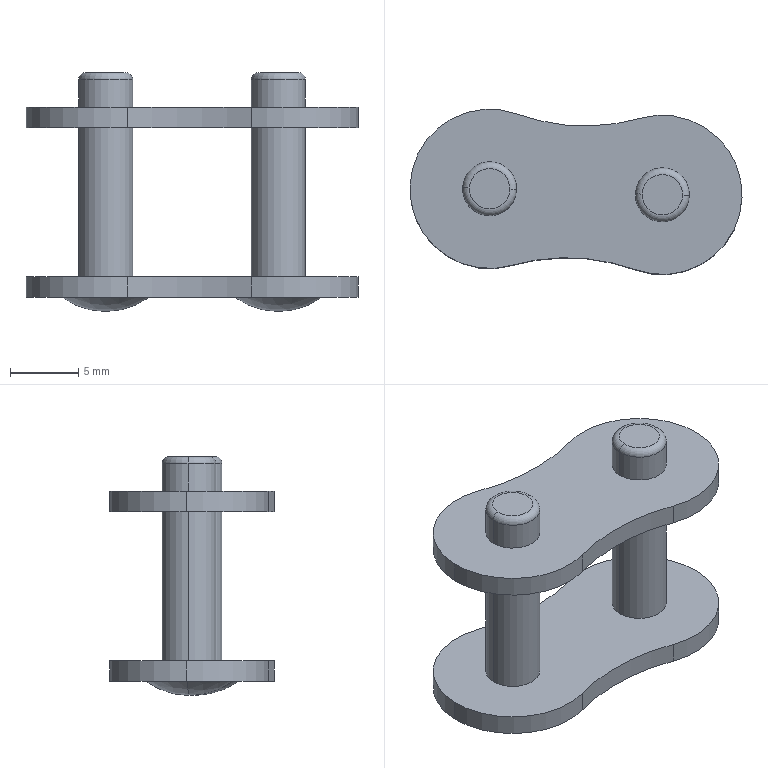Part | STEP file | CHES40-46-Part-10 | 1 solid | 32 faces | box 24.392 x 12.143 x 17.55 mm | volume 1093 mm3 | cylinder 18 | plane 6 | torus 4 | sphere 4 | commonest cylinder face diameters 3.97 x8 11.7 x6 29.64 x4
STEP:
#1=CARTESIAN_POINT('',(-138.255,-2.268,9.53));
#2=VERTEX_POINT('',#1);
#3=CARTESIAN_POINT('',(-141.223,-2.164,9.53));
#4=VERTEX_POINT('',#3);
#5=CARTESIAN_POINT('',(-139.739,-2.216,9.53));
#6=DIRECTION('',(0.,0.,1.));
#7=DIRECTION('',(-0.9994,0.0349,0.));
#8=AXIS2_PLACEMENT_3D('',#5,#6,#7);
#9=CIRCLE('',#8,1.485);
#10=EDGE_CURVE('',#2,#4,#9,.T.);
#11=ORIENTED_EDGE('',*,*,#10,.F.);
#12=CARTESIAN_POINT('',(-137.755,-2.285,9.03));
#13=VERTEX_POINT('',#12);
#14=CARTESIAN_POINT('',(-138.255,-2.268,9.03));
#15=DIRECTION('',(0.0349,0.9994,0.));
#16=DIRECTION('',(-0.9994,0.0349,0.));
#17=AXIS2_PLACEMENT_3D('',#14,#15,#16);
#18=CIRCLE('',#17,0.5);
#19=EDGE_CURVE('',#2,#13,#18,.T.);
#20=ORIENTED_EDGE('',*,*,#19,.T.);
#21=CARTESIAN_POINT('',(-141.722,-2.147,9.03));
#22=VERTEX_POINT('',#21);
#23=CARTESIAN_POINT('',(-139.739,-2.216,9.03));
#24=DIRECTION('',(0.,0.,-1.));
#25=DIRECTION('',(-0.9994,0.0349,0.));
#26=AXIS2_PLACEMENT_3D('',#23,#24,#25);
#27=CIRCLE('',#26,1.985);
#28=EDGE_CURVE('',#22,#13,#27,.T.);
#29=ORIENTED_EDGE('',*,*,#28,.F.);
#30=CARTESIAN_POINT('',(-141.223,-2.164,9.03));
#31=DIRECTION('',(-0.0349,-0.9994,0.));
#32=DIRECTION('',(0.9994,-0.0349,0.));
#33=AXIS2_PLACEMENT_3D('',#30,#31,#32);
#34=CIRCLE('',#33,0.5);
#35=EDGE_CURVE('',#4,#22,#34,.T.);
#36=ORIENTED_EDGE('',*,*,#35,.F.);
#37=EDGE_LOOP('',(#11,#20,#29,#36));
#38=FACE_OUTER_BOUND('',#37,.T.);
#39=CARTESIAN_POINT('',(-139.739,-2.216,9.03));
#40=DIRECTION('',(0.,0.,-1.));
#41=DIRECTION('',(-0.9994,0.0349,0.));
#42=AXIS2_PLACEMENT_3D('',#39,#40,#41);
#43=TOROIDAL_SURFACE('',#42,1.485,0.5);
#44=ADVANCED_FACE('',(#38),#43,.T.);
#45=CARTESIAN_POINT('',(-125.562,-2.711,9.53));
#46=VERTEX_POINT('',#45);
#47=CARTESIAN_POINT('',(-128.531,-2.608,9.53));
#48=VERTEX_POINT('',#47);
#49=CARTESIAN_POINT('',(-127.046,-2.659,9.53));
#50=DIRECTION('',(0.,0.,1.));
#51=DIRECTION('',(-0.9994,0.0349,0.));
#52=AXIS2_PLACEMENT_3D('',#49,#50,#51);
#53=CIRCLE('',#52,1.485);
#54=EDGE_CURVE('',#46,#48,#53,.T.);
#55=ORIENTED_EDGE('',*,*,#54,.F.);
#56=CARTESIAN_POINT('',(-125.063,-2.729,9.03));
#57=VERTEX_POINT('',#56);
#58=CARTESIAN_POINT('',(-125.562,-2.711,9.03));
#59=DIRECTION('',(0.0349,0.9994,0.));
#60=DIRECTION('',(-0.9994,0.0349,0.));
#61=AXIS2_PLACEMENT_3D('',#58,#59,#60);
#62=CIRCLE('',#61,0.5);
#63=EDGE_CURVE('',#46,#57,#62,.T.);
#64=ORIENTED_EDGE('',*,*,#63,.T.);
#65=CARTESIAN_POINT('',(-129.03,-2.59,9.03));
#66=VERTEX_POINT('',#65);
#67=CARTESIAN_POINT('',(-127.046,-2.659,9.03));
#68=DIRECTION('',(0.,0.,-1.));
#69=DIRECTION('',(-0.9994,0.0349,0.));
#70=AXIS2_PLACEMENT_3D('',#67,#68,#69);
#71=CIRCLE('',#70,1.985);
#72=EDGE_CURVE('',#66,#57,#71,.T.);
#73=ORIENTED_EDGE('',*,*,#72,.F.);
#74=CARTESIAN_POINT('',(-128.531,-2.608,9.03));
#75=DIRECTION('',(-0.0349,-0.9994,0.));
#76=DIRECTION('',(0.9994,-0.0349,0.));
#77=AXIS2_PLACEMENT_3D('',#74,#75,#76);
#78=CIRCLE('',#77,0.5);
#79=EDGE_CURVE('',#48,#66,#78,.T.);
#80=ORIENTED_EDGE('',*,*,#79,.F.);
#81=EDGE_LOOP('',(#55,#64,#73,#80));
#82=FACE_OUTER_BOUND('',#81,.T.);
#83=CARTESIAN_POINT('',(-127.046,-2.659,9.03));
#84=DIRECTION('',(0.,0.,-1.));
#85=DIRECTION('',(-0.9994,0.0349,0.));
#86=AXIS2_PLACEMENT_3D('',#83,#84,#85);
#87=TOROIDAL_SURFACE('',#86,1.485,0.5);
#88=ADVANCED_FACE('',(#82),#87,.T.);
#89=CARTESIAN_POINT('',(-142.937,-2.104,-6.975));
#90=VERTEX_POINT('',#89);
#91=CARTESIAN_POINT('',(-136.541,-2.328,-6.975));
#92=VERTEX_POINT('',#91);
#93=CARTESIAN_POINT('',(-139.739,-2.216,-6.975));
#94=DIRECTION('',(0.,0.,1.));
#95=DIRECTION('',(0.9994,-0.0349,0.));
#96=AXIS2_PLACEMENT_3D('',#93,#94,#95);
#97=CIRCLE('',#96,3.2);
#98=EDGE_CURVE('',#90,#92,#97,.T.);
#99=ORIENTED_EDGE('',*,*,#98,.F.);
#100=CARTESIAN_POINT('',(-139.739,-2.216,-8.02));
#101=VERTEX_POINT('',#100);
#102=CARTESIAN_POINT('',(-139.739,-2.216,-2.598));
#103=DIRECTION('',(-0.0349,-0.9994,0.));
#104=DIRECTION('',(0.9994,-0.0349,0.));
#105=AXIS2_PLACEMENT_3D('',#102,#103,#104);
#106=CIRCLE('',#105,5.422);
#107=EDGE_CURVE('',#90,#101,#106,.T.);
#108=ORIENTED_EDGE('',*,*,#107,.T.);
#109=CARTESIAN_POINT('',(-139.739,-2.216,-2.598));
#110=DIRECTION('',(0.0349,0.9994,0.));
#111=DIRECTION('',(-0.9994,0.0349,0.));
#112=AXIS2_PLACEMENT_3D('',#109,#110,#111);
#113=CIRCLE('',#112,5.422);
#114=EDGE_CURVE('',#92,#101,#113,.T.);
#115=ORIENTED_EDGE('',*,*,#114,.F.);
#116=EDGE_LOOP('',(#99,#108,#115));
#117=FACE_OUTER_BOUND('',#116,.T.);
#118=CARTESIAN_POINT('',(-139.739,-2.216,-2.598));
#119=DIRECTION('',(-0.0349,-0.9994,0.));
#120=DIRECTION('',(0.9994,-0.0349,0.));
#121=AXIS2_PLACEMENT_3D('',#118,#119,#120);
#122=SPHERICAL_SURFACE('',#121,5.422);
#123=ADVANCED_FACE('',(#117),#122,.T.);
#124=CARTESIAN_POINT('',(-130.244,-2.548,-6.975));
#125=VERTEX_POINT('',#124);
#126=CARTESIAN_POINT('',(-123.848,-2.771,-6.975));
#127=VERTEX_POINT('',#126);
#128=CARTESIAN_POINT('',(-127.046,-2.659,-6.975));
#129=DIRECTION('',(0.,0.,1.));
#130=DIRECTION('',(0.9994,-0.0349,0.));
#131=AXIS2_PLACEMENT_3D('',#128,#129,#130);
#132=CIRCLE('',#131,3.2);
#133=EDGE_CURVE('',#125,#127,#132,.T.);
#134=ORIENTED_EDGE('',*,*,#133,.F.);
#135=CARTESIAN_POINT('',(-127.046,-2.659,-8.02));
#136=VERTEX_POINT('',#135);
#137=CARTESIAN_POINT('',(-127.046,-2.659,-2.598));
#138=DIRECTION('',(-0.0349,-0.9994,0.));
#139=DIRECTION('',(0.9994,-0.0349,0.));
#140=AXIS2_PLACEMENT_3D('',#137,#138,#139);
#141=CIRCLE('',#140,5.422);
#142=EDGE_CURVE('',#125,#136,#141,.T.);
#143=ORIENTED_EDGE('',*,*,#142,.T.);
#144=CARTESIAN_POINT('',(-127.046,-2.659,-2.598));
#145=DIRECTION('',(0.0349,0.9994,0.));
#146=DIRECTION('',(-0.9994,0.0349,0.));
#147=AXIS2_PLACEMENT_3D('',#144,#145,#146);
#148=CIRCLE('',#147,5.422);
#149=EDGE_CURVE('',#127,#136,#148,.T.);
#150=ORIENTED_EDGE('',*,*,#149,.F.);
#151=EDGE_LOOP('',(#134,#143,#150));
#152=FACE_OUTER_BOUND('',#151,.T.);
#153=CARTESIAN_POINT('',(-127.046,-2.659,-2.598));
#154=DIRECTION('',(-0.0349,-0.9994,0.));
#155=DIRECTION('',(0.9994,-0.0349,0.));
#156=AXIS2_PLACEMENT_3D('',#153,#154,#155);
#157=SPHERICAL_SURFACE('',#156,5.422);
#158=ADVANCED_FACE('',(#152),#157,.T.);
#159=CARTESIAN_POINT('',(-145.585,-2.012,-5.475));
#160=VERTEX_POINT('',#159);
#161=CARTESIAN_POINT('',(-138.137,-7.843,-5.475));
#162=VERTEX_POINT('',#161);
#163=CARTESIAN_POINT('',(-139.739,-2.216,-5.475));
#164=DIRECTION('',(0.,0.,1.));
#165=DIRECTION('',(0.9994,-0.0349,0.));
#166=AXIS2_PLACEMENT_3D('',#163,#164,#165);
#167=CIRCLE('',#166,5.85);
#168=EDGE_CURVE('',#160,#162,#167,.T.);
#169=ORIENTED_EDGE('',*,*,#168,.F.);
#170=CARTESIAN_POINT('',(-145.585,-2.012,-6.975));
#171=VERTEX_POINT('',#170);
#172=CARTESIAN_POINT('',(-145.585,-2.012,-5.475));
#173=DIRECTION('',(0.,0.,-1.));
#174=VECTOR('',#173,1000.);
#175=LINE('',#172,#174);
#176=EDGE_CURVE('',#160,#171,#175,.T.);
#177=ORIENTED_EDGE('',*,*,#176,.T.);
#178=CARTESIAN_POINT('',(-138.137,-7.843,-6.975));
#179=VERTEX_POINT('',#178);
#180=CARTESIAN_POINT('',(-139.739,-2.216,-6.975));
#181=DIRECTION('',(0.,0.,1.));
#182=DIRECTION('',(0.9994,-0.0349,0.));
#183=AXIS2_PLACEMENT_3D('',#180,#181,#182);
#184=CIRCLE('',#183,5.85);
#185=EDGE_CURVE('',#171,#179,#184,.T.);
#186=ORIENTED_EDGE('',*,*,#185,.T.);
#187=CARTESIAN_POINT('',(-138.137,-7.843,-5.475));
#188=DIRECTION('',(0.,0.,-1.));
#189=VECTOR('',#188,1000.);
#190=LINE('',#187,#189);
#191=EDGE_CURVE('',#162,#179,#190,.T.);
#192=ORIENTED_EDGE('',*,*,#191,.F.);
#193=EDGE_LOOP('',(#169,#177,#186,#192));
#194=FACE_OUTER_BOUND('',#193,.T.);
#195=CARTESIAN_POINT('',(-139.739,-2.216,-5.475));
#196=DIRECTION('',(0.,0.,-1.));
#197=DIRECTION('',(-0.9994,0.0349,0.));
#198=AXIS2_PLACEMENT_3D('',#195,#196,#197);
#199=CYLINDRICAL_SURFACE('',#198,5.85);
#200=ADVANCED_FACE('',(#194),#199,.T.);
#201=CARTESIAN_POINT('',(-129.03,-2.59,5.475));
#202=VERTEX_POINT('',#201);
#203=CARTESIAN_POINT('',(-125.063,-2.729,5.475));
#204=VERTEX_POINT('',#203);
#205=CARTESIAN_POINT('',(-127.046,-2.659,5.475));
#206=DIRECTION('',(0.,0.,-1.));
#207=DIRECTION('',(-0.9994,0.0349,0.));
#208=AXIS2_PLACEMENT_3D('',#205,#206,#207);
#209=CIRCLE('',#208,1.985);
#210=EDGE_CURVE('',#202,#204,#209,.T.);
#211=ORIENTED_EDGE('',*,*,#210,.T.);
#212=CARTESIAN_POINT('',(-125.063,-2.729,-5.475));
#213=VERTEX_POINT('',#212);
#214=CARTESIAN_POINT('',(-125.063,-2.729,-8.02));
#215=DIRECTION('',(0.,0.,-1.));
#216=VECTOR('',#215,1000.);
#217=LINE('',#214,#216);
#218=EDGE_CURVE('',#204,#213,#217,.T.);
#219=ORIENTED_EDGE('',*,*,#218,.T.);
#220=CARTESIAN_POINT('',(-129.03,-2.59,-5.475));
#221=VERTEX_POINT('',#220);
#222=CARTESIAN_POINT('',(-127.046,-2.659,-5.475));
#223=DIRECTION('',(0.,0.,1.));
#224=DIRECTION('',(0.9994,-0.0349,0.));
#225=AXIS2_PLACEMENT_3D('',#222,#223,#224);
#226=CIRCLE('',#225,1.985);
#227=EDGE_CURVE('',#213,#221,#226,.T.);
#228=ORIENTED_EDGE('',*,*,#227,.T.);
#229=CARTESIAN_POINT('',(-129.03,-2.59,-8.02));
#230=DIRECTION('',(0.,0.,-1.));
#231=VECTOR('',#230,1000.);
#232=LINE('',#229,#231);
#233=EDGE_CURVE('',#202,#221,#232,.T.);
#234=ORIENTED_EDGE('',*,*,#233,.F.);
#235=EDGE_LOOP('',(#211,#219,#228,#234));
#236=FACE_OUTER_BOUND('',#235,.T.);
#237=CARTESIAN_POINT('',(-127.046,-2.659,-8.02));
#238=DIRECTION('',(0.,0.,-1.));
#239=DIRECTION('',(-0.9994,0.0349,0.));
#240=AXIS2_PLACEMENT_3D('',#237,#238,#239);
#241=CYLINDRICAL_SURFACE('',#240,1.985);
#242=ADVANCED_FACE('',(#236),#241,.T.);
#243=ORIENTED_EDGE('',*,*,#72,.T.);
#244=CARTESIAN_POINT('',(-125.063,-2.729,6.975));
#245=VERTEX_POINT('',#244);
#246=CARTESIAN_POINT('',(-125.063,-2.729,-8.02));
#247=DIRECTION('',(0.,0.,-1.));
#248=VECTOR('',#247,1000.);
#249=LINE('',#246,#248);
#250=EDGE_CURVE('',#57,#245,#249,.T.);
#251=ORIENTED_EDGE('',*,*,#250,.T.);
#252=CARTESIAN_POINT('',(-129.03,-2.59,6.975));
#253=VERTEX_POINT('',#252);
#254=CARTESIAN_POINT('',(-127.046,-2.659,6.975));
#255=DIRECTION('',(0.,0.,1.));
#256=DIRECTION('',(-0.9994,0.0349,0.));
#257=AXIS2_PLACEMENT_3D('',#254,#255,#256);
#258=CIRCLE('',#257,1.985);
#259=EDGE_CURVE('',#245,#253,#258,.T.);
#260=ORIENTED_EDGE('',*,*,#259,.T.);
#261=CARTESIAN_POINT('',(-129.03,-2.59,-8.02));
#262=DIRECTION('',(0.,0.,-1.));
#263=VECTOR('',#262,1000.);
#264=LINE('',#261,#263);
#265=EDGE_CURVE('',#66,#253,#264,.T.);
#266=ORIENTED_EDGE('',*,*,#265,.F.);
#267=EDGE_LOOP('',(#243,#251,#260,#266));
#268=FACE_OUTER_BOUND('',#267,.T.);
#269=CARTESIAN_POINT('',(-127.046,-2.659,-8.02));
#270=DIRECTION('',(0.,0.,-1.));
#271=DIRECTION('',(-0.9994,0.0349,0.));
#272=AXIS2_PLACEMENT_3D('',#269,#270,#271);
#273=CYLINDRICAL_SURFACE('',#272,1.985);
#274=ADVANCED_FACE('',(#268),#273,.T.);
#275=ORIENTED_EDGE('',*,*,#28,.T.);
#276=CARTESIAN_POINT('',(-137.755,-2.285,6.975));
#277=VERTEX_POINT('',#276);
#278=CARTESIAN_POINT('',(-137.755,-2.285,-8.02));
#279=DIRECTION('',(0.,0.,-1.));
#280=VECTOR('',#279,1000.);
#281=LINE('',#278,#280);
#282=EDGE_CURVE('',#13,#277,#281,.T.);
#283=ORIENTED_EDGE('',*,*,#282,.T.);
#284=CARTESIAN_POINT('',(-141.722,-2.147,6.975));
#285=VERTEX_POINT('',#284);
#286=CARTESIAN_POINT('',(-139.739,-2.216,6.975));
#287=DIRECTION('',(0.,0.,-1.));
#288=DIRECTION('',(-0.9994,0.0349,0.));
#289=AXIS2_PLACEMENT_3D('',#286,#287,#288);
#290=CIRCLE('',#289,1.985);
#291=EDGE_CURVE('',#285,#277,#290,.T.);
#292=ORIENTED_EDGE('',*,*,#291,.F.);
#293=CARTESIAN_POINT('',(-141.722,-2.147,-8.02));
#294=DIRECTION('',(0.,0.,-1.));
#295=VECTOR('',#294,1000.);
#296=LINE('',#293,#295);
#297=EDGE_CURVE('',#22,#285,#296,.T.);
#298=ORIENTED_EDGE('',*,*,#297,.F.);
#299=EDGE_LOOP('',(#275,#283,#292,#298));
#300=FACE_OUTER_BOUND('',#299,.T.);
#301=CARTESIAN_POINT('',(-139.739,-2.216,-8.02));
#302=DIRECTION('',(0.,0.,-1.));
#303=DIRECTION('',(-0.9994,0.0349,0.));
#304=AXIS2_PLACEMENT_3D('',#301,#302,#303);
#305=CYLINDRICAL_SURFACE('',#304,1.985);
#306=ADVANCED_FACE('',(#300),#305,.T.);
#307=CARTESIAN_POINT('',(-137.748,3.285,5.475));
#308=VERTEX_POINT('',#307);
#309=CARTESIAN_POINT('',(-145.585,-2.012,5.475));
#310=VERTEX_POINT('',#309);
#311=CARTESIAN_POINT('',(-139.739,-2.216,5.475));
#312=DIRECTION('',(0.,0.,1.));
#313=DIRECTION('',(0.9994,-0.0349,0.));
#314=AXIS2_PLACEMENT_3D('',#311,#312,#313);
#315=CIRCLE('',#314,5.85);
#316=EDGE_CURVE('',#308,#310,#315,.T.);
#317=ORIENTED_EDGE('',*,*,#316,.T.);
#318=CARTESIAN_POINT('',(-145.585,-2.012,6.975));
#319=VERTEX_POINT('',#318);
#320=CARTESIAN_POINT('',(-145.585,-2.012,5.475));
#321=DIRECTION('',(0.,0.,1.));
#322=VECTOR('',#321,1000.);
#323=LINE('',#320,#322);
#324=EDGE_CURVE('',#310,#319,#323,.T.);
#325=ORIENTED_EDGE('',*,*,#324,.T.);
#326=CARTESIAN_POINT('',(-137.748,3.285,6.975));
#327=VERTEX_POINT('',#326);
#328=CARTESIAN_POINT('',(-139.739,-2.216,6.975));
#329=DIRECTION('',(0.,0.,1.));
#330=DIRECTION('',(0.9994,-0.0349,0.));
#331=AXIS2_PLACEMENT_3D('',#328,#329,#330);
#332=CIRCLE('',#331,5.85);
#333=EDGE_CURVE('',#327,#319,#332,.T.);
#334=ORIENTED_EDGE('',*,*,#333,.F.);
#335=CARTESIAN_POINT('',(-137.748,3.285,5.475));
#336=DIRECTION('',(0.,0.,1.));
#337=VECTOR('',#336,1000.);
#338=LINE('',#335,#337);
#339=EDGE_CURVE('',#308,#327,#338,.T.);
#340=ORIENTED_EDGE('',*,*,#339,.F.);
#341=EDGE_LOOP('',(#317,#325,#334,#340));
#342=FACE_OUTER_BOUND('',#341,.T.);
#343=CARTESIAN_POINT('',(-139.739,-2.216,5.475));
#344=DIRECTION('',(0.,0.,1.));
#345=DIRECTION('',(-0.9994,0.0349,0.));
#346=AXIS2_PLACEMENT_3D('',#343,#344,#345);
#347=CYLINDRICAL_SURFACE('',#346,5.85);
#348=ADVANCED_FACE('',(#342),#347,.T.);
#349=CARTESIAN_POINT('',(-141.722,-2.147,5.475));
#350=VERTEX_POINT('',#349);
#351=CARTESIAN_POINT('',(-137.755,-2.285,5.475));
#352=VERTEX_POINT('',#351);
#353=CARTESIAN_POINT('',(-139.739,-2.216,5.475));
#354=DIRECTION('',(0.,0.,-1.));
#355=DIRECTION('',(-0.9994,0.0349,0.));
#356=AXIS2_PLACEMENT_3D('',#353,#354,#355);
#357=CIRCLE('',#356,1.985);
#358=EDGE_CURVE('',#350,#352,#357,.T.);
#359=ORIENTED_EDGE('',*,*,#358,.T.);
#360=CARTESIAN_POINT('',(-137.755,-2.285,-5.475));
#361=VERTEX_POINT('',#360);
#362=CARTESIAN_POINT('',(-137.755,-2.285,-8.02));
#363=DIRECTION('',(0.,0.,-1.));
#364=VECTOR('',#363,1000.);
#365=LINE('',#362,#364);
#366=EDGE_CURVE('',#352,#361,#365,.T.);
#367=ORIENTED_EDGE('',*,*,#366,.T.);
#368=CARTESIAN_POINT('',(-141.722,-2.147,-5.475));
#369=VERTEX_POINT('',#368);
#370=CARTESIAN_POINT('',(-139.739,-2.216,-5.475));
#371=DIRECTION('',(0.,0.,1.));
#372=DIRECTION('',(0.9994,-0.0349,0.));
#373=AXIS2_PLACEMENT_3D('',#370,#371,#372);
#374=CIRCLE('',#373,1.985);
#375=EDGE_CURVE('',#361,#369,#374,.T.);
#376=ORIENTED_EDGE('',*,*,#375,.T.);
#377=CARTESIAN_POINT('',(-141.722,-2.147,-8.02));
#378=DIRECTION('',(0.,0.,-1.));
#379=VECTOR('',#378,1000.);
#380=LINE('',#377,#379);
#381=EDGE_CURVE('',#350,#369,#380,.T.);
#382=ORIENTED_EDGE('',*,*,#381,.F.);
#383=EDGE_LOOP('',(#359,#367,#376,#382));
#384=FACE_OUTER_BOUND('',#383,.T.);
#385=CARTESIAN_POINT('',(-139.739,-2.216,-8.02));
#386=DIRECTION('',(0.,0.,-1.));
#387=DIRECTION('',(-0.9994,0.0349,0.));
#388=AXIS2_PLACEMENT_3D('',#385,#386,#387);
#389=CYLINDRICAL_SURFACE('',#388,1.985);
#390=ADVANCED_FACE('',(#384),#389,.T.);
#391=ORIENTED_EDGE('',*,*,#358,.F.);
#392=CARTESIAN_POINT('',(-139.739,-2.216,5.475));
#393=DIRECTION('',(0.,0.,-1.));
#394=DIRECTION('',(-0.9994,0.0349,0.));
#395=AXIS2_PLACEMENT_3D('',#392,#393,#394);
#396=CIRCLE('',#395,1.985);
#397=EDGE_CURVE('',#352,#350,#396,.T.);
#398=ORIENTED_EDGE('',*,*,#397,.F.);
#399=EDGE_LOOP('',(#391,#398));
#400=FACE_BOUND('',#399,.T.);
#401=ORIENTED_EDGE('',*,*,#316,.F.);
#402=CARTESIAN_POINT('',(-128.648,2.967,5.475));
#403=VERTEX_POINT('',#402);
#404=CARTESIAN_POINT('',(-132.706,17.221,5.475));
#405=DIRECTION('',(0.,0.,-1.));
#406=DIRECTION('',(0.9994,-0.0349,0.));
#407=AXIS2_PLACEMENT_3D('',#404,#405,#406);
#408=CIRCLE('',#407,14.82);
#409=EDGE_CURVE('',#403,#308,#408,.T.);
#410=ORIENTED_EDGE('',*,*,#409,.F.);
#411=CARTESIAN_POINT('',(-129.037,-8.16,5.475));
#412=VERTEX_POINT('',#411);
#413=CARTESIAN_POINT('',(-127.046,-2.659,5.475));
#414=DIRECTION('',(0.,0.,1.));
#415=DIRECTION('',(-0.9994,0.0349,0.));
#416=AXIS2_PLACEMENT_3D('',#413,#414,#415);
#417=CIRCLE('',#416,5.85);
#418=EDGE_CURVE('',#412,#403,#417,.T.);
#419=ORIENTED_EDGE('',*,*,#418,.F.);
#420=CARTESIAN_POINT('',(-138.137,-7.843,5.475));
#421=VERTEX_POINT('',#420);
#422=CARTESIAN_POINT('',(-134.079,-22.096,5.475));
#423=DIRECTION('',(0.,0.,-1.));
#424=DIRECTION('',(-0.9994,0.0349,0.));
#425=AXIS2_PLACEMENT_3D('',#422,#423,#424);
#426=CIRCLE('',#425,14.82);
#427=EDGE_CURVE('',#421,#412,#426,.T.);
#428=ORIENTED_EDGE('',*,*,#427,.F.);
#429=CARTESIAN_POINT('',(-139.739,-2.216,5.475));
#430=DIRECTION('',(0.,0.,1.));
#431=DIRECTION('',(0.9994,-0.0349,0.));
#432=AXIS2_PLACEMENT_3D('',#429,#430,#431);
#433=CIRCLE('',#432,5.85);
#434=EDGE_CURVE('',#310,#421,#433,.T.);
#435=ORIENTED_EDGE('',*,*,#434,.F.);
#436=EDGE_LOOP('',(#401,#410,#419,#428,#435));
#437=FACE_OUTER_BOUND('',#436,.T.);
#438=ORIENTED_EDGE('',*,*,#210,.F.);
#439=CARTESIAN_POINT('',(-127.046,-2.659,5.475));
#440=DIRECTION('',(0.,0.,-1.));
#441=DIRECTION('',(-0.9994,0.0349,0.));
#442=AXIS2_PLACEMENT_3D('',#439,#440,#441);
#443=CIRCLE('',#442,1.985);
#444=EDGE_CURVE('',#204,#202,#443,.T.);
#445=ORIENTED_EDGE('',*,*,#444,.F.);
#446=EDGE_LOOP('',(#438,#445));
#447=FACE_BOUND('',#446,.T.);
#448=CARTESIAN_POINT('',(-136.909,-12.156,5.475));
#449=DIRECTION('',(0.,0.,-1.));
#450=DIRECTION('',(0.9994,-0.0349,0.));
#451=AXIS2_PLACEMENT_3D('',#448,#449,#450);
#452=PLANE('',#451);
#453=ADVANCED_FACE('',(#400,#437,#447),#452,.T.);
#454=ORIENTED_EDGE('',*,*,#366,.F.);
#455=ORIENTED_EDGE('',*,*,#397,.T.);
#456=ORIENTED_EDGE('',*,*,#381,.T.);
#457=CARTESIAN_POINT('',(-139.739,-2.216,-5.475));
#458=DIRECTION('',(0.,0.,1.));
#459=DIRECTION('',(0.9994,-0.0349,0.));
#460=AXIS2_PLACEMENT_3D('',#457,#458,#459);
#461=CIRCLE('',#460,1.985);
#462=EDGE_CURVE('',#369,#361,#461,.T.);
#463=ORIENTED_EDGE('',*,*,#462,.T.);
#464=EDGE_LOOP('',(#454,#455,#456,#463));
#465=FACE_OUTER_BOUND('',#464,.T.);
#466=CARTESIAN_POINT('',(-139.739,-2.216,-8.02));
#467=DIRECTION('',(0.,0.,-1.));
#468=DIRECTION('',(-0.9994,0.0349,0.));
#469=AXIS2_PLACEMENT_3D('',#466,#467,#468);
#470=CYLINDRICAL_SURFACE('',#469,1.985);
#471=ADVANCED_FACE('',(#465),#470,.T.);
#472=CARTESIAN_POINT('',(-127.046,-2.659,6.975));
#473=DIRECTION('',(0.,0.,1.));
#474=DIRECTION('',(-0.9994,0.0349,0.));
#475=AXIS2_PLACEMENT_3D('',#472,#473,#474);
#476=CIRCLE('',#475,1.985);
#477=EDGE_CURVE('',#253,#245,#476,.T.);
#478=ORIENTED_EDGE('',*,*,#477,.F.);
#479=ORIENTED_EDGE('',*,*,#259,.F.);
#480=EDGE_LOOP('',(#478,#479));
#481=FACE_BOUND('',#480,.T.);
#482=ORIENTED_EDGE('',*,*,#333,.T.);
#483=CARTESIAN_POINT('',(-138.137,-7.843,6.975));
#484=VERTEX_POINT('',#483);
#485=CARTESIAN_POINT('',(-139.739,-2.216,6.975));
#486=DIRECTION('',(0.,0.,1.));
#487=DIRECTION('',(0.9994,-0.0349,0.));
#488=AXIS2_PLACEMENT_3D('',#485,#486,#487);
#489=CIRCLE('',#488,5.85);
#490=EDGE_CURVE('',#319,#484,#489,.T.);
#491=ORIENTED_EDGE('',*,*,#490,.T.);
#492=CARTESIAN_POINT('',(-129.037,-8.16,6.975));
#493=VERTEX_POINT('',#492);
#494=CARTESIAN_POINT('',(-134.079,-22.096,6.975));
#495=DIRECTION('',(0.,0.,-1.));
#496=DIRECTION('',(-0.9994,0.0349,0.));
#497=AXIS2_PLACEMENT_3D('',#494,#495,#496);
#498=CIRCLE('',#497,14.82);
#499=EDGE_CURVE('',#484,#493,#498,.T.);
#500=ORIENTED_EDGE('',*,*,#499,.T.);
#501=CARTESIAN_POINT('',(-128.648,2.967,6.975));
#502=VERTEX_POINT('',#501);
#503=CARTESIAN_POINT('',(-127.046,-2.659,6.975));
#504=DIRECTION('',(0.,0.,1.));
#505=DIRECTION('',(-0.9994,0.0349,0.));
#506=AXIS2_PLACEMENT_3D('',#503,#504,#505);
#507=CIRCLE('',#506,5.85);
#508=EDGE_CURVE('',#493,#502,#507,.T.);
#509=ORIENTED_EDGE('',*,*,#508,.T.);
#510=CARTESIAN_POINT('',(-132.706,17.221,6.975));
#511=DIRECTION('',(0.,0.,-1.));
#512=DIRECTION('',(0.9994,-0.0349,0.));
#513=AXIS2_PLACEMENT_3D('',#510,#511,#512);
#514=CIRCLE('',#513,14.82);
#515=EDGE_CURVE('',#502,#327,#514,.T.);
#516=ORIENTED_EDGE('',*,*,#515,.T.);
#517=EDGE_LOOP('',(#482,#491,#500,#509,#516));
#518=FACE_OUTER_BOUND('',#517,.T.);
#519=ORIENTED_EDGE('',*,*,#291,.T.);
#520=CARTESIAN_POINT('',(-139.739,-2.216,6.975));
#521=DIRECTION('',(0.,0.,-1.));
#522=DIRECTION('',(-0.9994,0.0349,0.));
#523=AXIS2_PLACEMENT_3D('',#520,#521,#522);
#524=CIRCLE('',#523,1.985);
#525=EDGE_CURVE('',#277,#285,#524,.T.);
#526=ORIENTED_EDGE('',*,*,#525,.T.);
#527=EDGE_LOOP('',(#519,#526));
#528=FACE_BOUND('',#527,.T.);
#529=CARTESIAN_POINT('',(-136.909,-12.156,6.975));
#530=DIRECTION('',(0.,0.,-1.));
#531=DIRECTION('',(0.9994,-0.0349,0.));
#532=AXIS2_PLACEMENT_3D('',#529,#530,#531);
#533=PLANE('',#532);
#534=ADVANCED_FACE('',(#481,#518,#528),#533,.F.);
#535=ORIENTED_EDGE('',*,*,#324,.F.);
#536=ORIENTED_EDGE('',*,*,#434,.T.);
#537=CARTESIAN_POINT('',(-138.137,-7.843,5.475));
#538=DIRECTION('',(0.,0.,1.));
#539=VECTOR('',#538,1000.);
#540=LINE('',#537,#539);
#541=EDGE_CURVE('',#421,#484,#540,.T.);
#542=ORIENTED_EDGE('',*,*,#541,.T.);
#543=ORIENTED_EDGE('',*,*,#490,.F.);
#544=EDGE_LOOP('',(#535,#536,#542,#543));
#545=FACE_OUTER_BOUND('',#544,.T.);
#546=CARTESIAN_POINT('',(-139.739,-2.216,5.475));
#547=DIRECTION('',(0.,0.,1.));
#548=DIRECTION('',(-0.9994,0.0349,0.));
#549=AXIS2_PLACEMENT_3D('',#546,#547,#548);
#550=CYLINDRICAL_SURFACE('',#549,5.85);
#551=ADVANCED_FACE('',(#545),#550,.T.);
#552=ORIENTED_EDGE('',*,*,#499,.F.);
#553=ORIENTED_EDGE('',*,*,#541,.F.);
#554=ORIENTED_EDGE('',*,*,#427,.T.);
#555=CARTESIAN_POINT('',(-129.037,-8.16,5.475));
#556=DIRECTION('',(0.,0.,1.));
#557=VECTOR('',#556,1000.);
#558=LINE('',#555,#557);
#559=EDGE_CURVE('',#412,#493,#558,.T.);
#560=ORIENTED_EDGE('',*,*,#559,.T.);
#561=EDGE_LOOP('',(#552,#553,#554,#560));
#562=FACE_OUTER_BOUND('',#561,.T.);
#563=CARTESIAN_POINT('',(-134.079,-22.096,5.475));
#564=DIRECTION('',(0.,0.,1.));
#565=DIRECTION('',(-0.9994,0.0349,0.));
#566=AXIS2_PLACEMENT_3D('',#563,#564,#565);
#567=CYLINDRICAL_SURFACE('',#566,14.82);
#568=ADVANCED_FACE('',(#562),#567,.F.);
#569=ORIENTED_EDGE('',*,*,#508,.F.);
#570=ORIENTED_EDGE('',*,*,#559,.F.);
#571=ORIENTED_EDGE('',*,*,#418,.T.);
#572=CARTESIAN_POINT('',(-128.648,2.967,5.475));
#573=DIRECTION('',(0.,0.,1.));
#574=VECTOR('',#573,1000.);
#575=LINE('',#572,#574);
#576=EDGE_CURVE('',#403,#502,#575,.T.);
#577=ORIENTED_EDGE('',*,*,#576,.T.);
#578=EDGE_LOOP('',(#569,#570,#571,#577));
#579=FACE_OUTER_BOUND('',#578,.T.);
#580=CARTESIAN_POINT('',(-127.046,-2.659,5.475));
#581=DIRECTION('',(0.,0.,1.));
#582=DIRECTION('',(-0.9994,0.0349,0.));
#583=AXIS2_PLACEMENT_3D('',#580,#581,#582);
#584=CYLINDRICAL_SURFACE('',#583,5.85);
#585=ADVANCED_FACE('',(#579),#584,.T.);
#586=ORIENTED_EDGE('',*,*,#515,.F.);
#587=ORIENTED_EDGE('',*,*,#576,.F.);
#588=ORIENTED_EDGE('',*,*,#409,.T.);
#589=ORIENTED_EDGE('',*,*,#339,.T.);
#590=EDGE_LOOP('',(#586,#587,#588,#589));
#591=FACE_OUTER_BOUND('',#590,.T.);
#592=CARTESIAN_POINT('',(-132.706,17.221,5.475));
#593=DIRECTION('',(0.,0.,1.));
#594=DIRECTION('',(-0.9994,0.0349,0.));
#595=AXIS2_PLACEMENT_3D('',#592,#593,#594);
#596=CYLINDRICAL_SURFACE('',#595,14.82);
#597=ADVANCED_FACE('',(#591),#596,.F.);
#598=CARTESIAN_POINT('',(-139.739,-2.216,9.53));
#599=DIRECTION('',(0.,0.,1.));
#600=DIRECTION('',(-0.9994,0.0349,0.));
#601=AXIS2_PLACEMENT_3D('',#598,#599,#600);
#602=CIRCLE('',#601,1.485);
#603=EDGE_CURVE('',#4,#2,#602,.T.);
#604=ORIENTED_EDGE('',*,*,#603,.T.);
#605=ORIENTED_EDGE('',*,*,#10,.T.);
#606=EDGE_LOOP('',(#604,#605));
#607=FACE_OUTER_BOUND('',#606,.T.);
#608=CARTESIAN_POINT('',(-137.755,-2.285,9.53));
#609=DIRECTION('',(0.,0.,-1.));
#610=DIRECTION('',(-0.9994,0.0349,0.));
#611=AXIS2_PLACEMENT_3D('',#608,#609,#610);
#612=PLANE('',#611);
#613=ADVANCED_FACE('',(#607),#612,.F.);
#614=ORIENTED_EDGE('',*,*,#282,.F.);
#615=CARTESIAN_POINT('',(-139.739,-2.216,9.03));
#616=DIRECTION('',(0.,0.,-1.));
#617=DIRECTION('',(-0.9994,0.0349,0.));
#618=AXIS2_PLACEMENT_3D('',#615,#616,#617);
#619=CIRCLE('',#618,1.985);
#620=EDGE_CURVE('',#13,#22,#619,.T.);
#621=ORIENTED_EDGE('',*,*,#620,.T.);
#622=ORIENTED_EDGE('',*,*,#297,.T.);
#623=ORIENTED_EDGE('',*,*,#525,.F.);
#624=EDGE_LOOP('',(#614,#621,#622,#623));
#625=FACE_OUTER_BOUND('',#624,.T.);
#626=CARTESIAN_POINT('',(-139.739,-2.216,-8.02));
#627=DIRECTION('',(0.,0.,-1.));
#628=DIRECTION('',(-0.9994,0.0349,0.));
#629=AXIS2_PLACEMENT_3D('',#626,#627,#628);
#630=CYLINDRICAL_SURFACE('',#629,1.985);
#631=ADVANCED_FACE('',(#625),#630,.T.);
#632=CARTESIAN_POINT('',(-127.046,-2.659,9.53));
#633=DIRECTION('',(0.,0.,1.));
#634=DIRECTION('',(-0.9994,0.0349,0.));
#635=AXIS2_PLACEMENT_3D('',#632,#633,#634);
#636=CIRCLE('',#635,1.485);
#637=EDGE_CURVE('',#48,#46,#636,.T.);
#638=ORIENTED_EDGE('',*,*,#637,.T.);
#639=ORIENTED_EDGE('',*,*,#54,.T.);
#640=EDGE_LOOP('',(#638,#639));
#641=FACE_OUTER_BOUND('',#640,.T.);
#642=CARTESIAN_POINT('',(-127.046,-2.659,9.53));
#643=DIRECTION('',(0.,0.,-1.));
#644=DIRECTION('',(-0.9994,0.0349,0.));
#645=AXIS2_PLACEMENT_3D('',#642,#643,#644);
#646=PLANE('',#645);
#647=ADVANCED_FACE('',(#641),#646,.F.);
#648=ORIENTED_EDGE('',*,*,#250,.F.);
#649=CARTESIAN_POINT('',(-127.046,-2.659,9.03));
#650=DIRECTION('',(0.,0.,-1.));
#651=DIRECTION('',(-0.9994,0.0349,0.));
#652=AXIS2_PLACEMENT_3D('',#649,#650,#651);
#653=CIRCLE('',#652,1.985);
#654=EDGE_CURVE('',#57,#66,#653,.T.);
#655=ORIENTED_EDGE('',*,*,#654,.T.);
#656=ORIENTED_EDGE('',*,*,#265,.T.);
#657=ORIENTED_EDGE('',*,*,#477,.T.);
#658=EDGE_LOOP('',(#648,#655,#656,#657));
#659=FACE_OUTER_BOUND('',#658,.T.);
#660=CARTESIAN_POINT('',(-127.046,-2.659,-8.02));
#661=DIRECTION('',(0.,0.,-1.));
#662=DIRECTION('',(-0.9994,0.0349,0.));
#663=AXIS2_PLACEMENT_3D('',#660,#661,#662);
#664=CYLINDRICAL_SURFACE('',#663,1.985);
#665=ADVANCED_FACE('',(#659),#664,.T.);
#666=ORIENTED_EDGE('',*,*,#218,.F.);
#667=ORIENTED_EDGE('',*,*,#444,.T.);
#668=ORIENTED_EDGE('',*,*,#233,.T.);
#669=CARTESIAN_POINT('',(-127.046,-2.659,-5.475));
#670=DIRECTION('',(0.,0.,1.));
#671=DIRECTION('',(0.9994,-0.0349,0.));
#672=AXIS2_PLACEMENT_3D('',#669,#670,#671);
#673=CIRCLE('',#672,1.985);
#674=EDGE_CURVE('',#221,#213,#673,.T.);
#675=ORIENTED_EDGE('',*,*,#674,.T.);
#676=EDGE_LOOP('',(#666,#667,#668,#675));
#677=FACE_OUTER_BOUND('',#676,.T.);
#678=CARTESIAN_POINT('',(-127.046,-2.659,-8.02));
#679=DIRECTION('',(0.,0.,-1.));
#680=DIRECTION('',(-0.9994,0.0349,0.));
#681=AXIS2_PLACEMENT_3D('',#678,#679,#680);
#682=CYLINDRICAL_SURFACE('',#681,1.985);
#683=ADVANCED_FACE('',(#677),#682,.T.);
#684=CARTESIAN_POINT('',(-137.748,3.285,-5.475));
#685=VERTEX_POINT('',#684);
#686=CARTESIAN_POINT('',(-139.739,-2.216,-5.475));
#687=DIRECTION('',(0.,0.,1.));
#688=DIRECTION('',(0.9994,-0.0349,0.));
#689=AXIS2_PLACEMENT_3D('',#686,#687,#688);
#690=CIRCLE('',#689,5.85);
#691=EDGE_CURVE('',#685,#160,#690,.T.);
#692=ORIENTED_EDGE('',*,*,#691,.T.);
#693=ORIENTED_EDGE('',*,*,#168,.T.);
#694=CARTESIAN_POINT('',(-129.037,-8.16,-5.475));
#695=VERTEX_POINT('',#694);
#696=CARTESIAN_POINT('',(-134.079,-22.096,-5.475));
#697=DIRECTION('',(0.,0.,-1.));
#698=DIRECTION('',(-0.9994,0.0349,0.));
#699=AXIS2_PLACEMENT_3D('',#696,#697,#698);
#700=CIRCLE('',#699,14.82);
#701=EDGE_CURVE('',#162,#695,#700,.T.);
#702=ORIENTED_EDGE('',*,*,#701,.T.);
#703=CARTESIAN_POINT('',(-128.648,2.967,-5.475));
#704=VERTEX_POINT('',#703);
#705=CARTESIAN_POINT('',(-127.046,-2.659,-5.475));
#706=DIRECTION('',(0.,0.,1.));
#707=DIRECTION('',(-0.9994,0.0349,0.));
#708=AXIS2_PLACEMENT_3D('',#705,#706,#707);
#709=CIRCLE('',#708,5.85);
#710=EDGE_CURVE('',#695,#704,#709,.T.);
#711=ORIENTED_EDGE('',*,*,#710,.T.);
#712=CARTESIAN_POINT('',(-132.706,17.221,-5.475));
#713=DIRECTION('',(0.,0.,-1.));
#714=DIRECTION('',(0.9994,-0.0349,0.));
#715=AXIS2_PLACEMENT_3D('',#712,#713,#714);
#716=CIRCLE('',#715,14.82);
#717=EDGE_CURVE('',#704,#685,#716,.T.);
#718=ORIENTED_EDGE('',*,*,#717,.T.);
#719=EDGE_LOOP('',(#692,#693,#702,#711,#718));
#720=FACE_OUTER_BOUND('',#719,.T.);
#721=ORIENTED_EDGE('',*,*,#674,.F.);
#722=ORIENTED_EDGE('',*,*,#227,.F.);
#723=EDGE_LOOP('',(#721,#722));
#724=FACE_BOUND('',#723,.T.);
#725=ORIENTED_EDGE('',*,*,#462,.F.);
#726=ORIENTED_EDGE('',*,*,#375,.F.);
#727=EDGE_LOOP('',(#725,#726));
#728=FACE_BOUND('',#727,.T.);
#729=CARTESIAN_POINT('',(-136.909,-12.156,-5.475));
#730=DIRECTION('',(0.,0.,1.));
#731=DIRECTION('',(0.9994,-0.0349,0.));
#732=AXIS2_PLACEMENT_3D('',#729,#730,#731);
#733=PLANE('',#732);
#734=ADVANCED_FACE('',(#720,#724,#728),#733,.T.);
#735=CARTESIAN_POINT('',(-137.748,3.285,-6.975));
#736=VERTEX_POINT('',#735);
#737=CARTESIAN_POINT('',(-139.739,-2.216,-6.975));
#738=DIRECTION('',(0.,0.,1.));
#739=DIRECTION('',(0.9994,-0.0349,0.));
#740=AXIS2_PLACEMENT_3D('',#737,#738,#739);
#741=CIRCLE('',#740,5.85);
#742=EDGE_CURVE('',#736,#171,#741,.T.);
#743=ORIENTED_EDGE('',*,*,#742,.F.);
#744=CARTESIAN_POINT('',(-128.648,2.967,-6.975));
#745=VERTEX_POINT('',#744);
#746=CARTESIAN_POINT('',(-132.706,17.221,-6.975));
#747=DIRECTION('',(0.,0.,-1.));
#748=DIRECTION('',(0.9994,-0.0349,0.));
#749=AXIS2_PLACEMENT_3D('',#746,#747,#748);
#750=CIRCLE('',#749,14.82);
#751=EDGE_CURVE('',#745,#736,#750,.T.);
#752=ORIENTED_EDGE('',*,*,#751,.F.);
#753=CARTESIAN_POINT('',(-129.037,-8.16,-6.975));
#754=VERTEX_POINT('',#753);
#755=CARTESIAN_POINT('',(-127.046,-2.659,-6.975));
#756=DIRECTION('',(0.,0.,1.));
#757=DIRECTION('',(-0.9994,0.0349,0.));
#758=AXIS2_PLACEMENT_3D('',#755,#756,#757);
#759=CIRCLE('',#758,5.85);
#760=EDGE_CURVE('',#754,#745,#759,.T.);
#761=ORIENTED_EDGE('',*,*,#760,.F.);
#762=CARTESIAN_POINT('',(-134.079,-22.096,-6.975));
#763=DIRECTION('',(0.,0.,-1.));
#764=DIRECTION('',(-0.9994,0.0349,0.));
#765=AXIS2_PLACEMENT_3D('',#762,#763,#764);
#766=CIRCLE('',#765,14.82);
#767=EDGE_CURVE('',#179,#754,#766,.T.);
#768=ORIENTED_EDGE('',*,*,#767,.F.);
#769=ORIENTED_EDGE('',*,*,#185,.F.);
#770=EDGE_LOOP('',(#743,#752,#761,#768,#769));
#771=FACE_OUTER_BOUND('',#770,.T.);
#772=CARTESIAN_POINT('',(-127.046,-2.659,-6.975));
#773=DIRECTION('',(0.,0.,1.));
#774=DIRECTION('',(0.9994,-0.0349,0.));
#775=AXIS2_PLACEMENT_3D('',#772,#773,#774);
#776=CIRCLE('',#775,3.2);
#777=EDGE_CURVE('',#127,#125,#776,.T.);
#778=ORIENTED_EDGE('',*,*,#777,.T.);
#779=ORIENTED_EDGE('',*,*,#133,.T.);
#780=EDGE_LOOP('',(#778,#779));
#781=FACE_BOUND('',#780,.T.);
#782=CARTESIAN_POINT('',(-139.739,-2.216,-6.975));
#783=DIRECTION('',(0.,0.,1.));
#784=DIRECTION('',(0.9994,-0.0349,0.));
#785=AXIS2_PLACEMENT_3D('',#782,#783,#784);
#786=CIRCLE('',#785,3.2);
#787=EDGE_CURVE('',#92,#90,#786,.T.);
#788=ORIENTED_EDGE('',*,*,#787,.T.);
#789=ORIENTED_EDGE('',*,*,#98,.T.);
#790=EDGE_LOOP('',(#788,#789));
#791=FACE_BOUND('',#790,.T.);
#792=CARTESIAN_POINT('',(-136.909,-12.156,-6.975));
#793=DIRECTION('',(0.,0.,1.));
#794=DIRECTION('',(0.9994,-0.0349,0.));
#795=AXIS2_PLACEMENT_3D('',#792,#793,#794);
#796=PLANE('',#795);
#797=ADVANCED_FACE('',(#771,#781,#791),#796,.F.);
#798=ORIENTED_EDGE('',*,*,#176,.F.);
#799=ORIENTED_EDGE('',*,*,#691,.F.);
#800=CARTESIAN_POINT('',(-137.748,3.285,-5.475));
#801=DIRECTION('',(0.,0.,-1.));
#802=VECTOR('',#801,1000.);
#803=LINE('',#800,#802);
#804=EDGE_CURVE('',#685,#736,#803,.T.);
#805=ORIENTED_EDGE('',*,*,#804,.T.);
#806=ORIENTED_EDGE('',*,*,#742,.T.);
#807=EDGE_LOOP('',(#798,#799,#805,#806));
#808=FACE_OUTER_BOUND('',#807,.T.);
#809=CARTESIAN_POINT('',(-139.739,-2.216,-5.475));
#810=DIRECTION('',(0.,0.,-1.));
#811=DIRECTION('',(-0.9994,0.0349,0.));
#812=AXIS2_PLACEMENT_3D('',#809,#810,#811);
#813=CYLINDRICAL_SURFACE('',#812,5.85);
#814=ADVANCED_FACE('',(#808),#813,.T.);
#815=ORIENTED_EDGE('',*,*,#767,.T.);
#816=CARTESIAN_POINT('',(-129.037,-8.16,-5.475));
#817=DIRECTION('',(0.,0.,-1.));
#818=VECTOR('',#817,1000.);
#819=LINE('',#816,#818);
#820=EDGE_CURVE('',#695,#754,#819,.T.);
#821=ORIENTED_EDGE('',*,*,#820,.F.);
#822=ORIENTED_EDGE('',*,*,#701,.F.);
#823=ORIENTED_EDGE('',*,*,#191,.T.);
#824=EDGE_LOOP('',(#815,#821,#822,#823));
#825=FACE_OUTER_BOUND('',#824,.T.);
#826=CARTESIAN_POINT('',(-134.079,-22.096,-5.475));
#827=DIRECTION('',(0.,0.,-1.));
#828=DIRECTION('',(-0.9994,0.0349,0.));
#829=AXIS2_PLACEMENT_3D('',#826,#827,#828);
#830=CYLINDRICAL_SURFACE('',#829,14.82);
#831=ADVANCED_FACE('',(#825),#830,.F.);
#832=ORIENTED_EDGE('',*,*,#760,.T.);
#833=CARTESIAN_POINT('',(-128.648,2.967,-5.475));
#834=DIRECTION('',(0.,0.,-1.));
#835=VECTOR('',#834,1000.);
#836=LINE('',#833,#835);
#837=EDGE_CURVE('',#704,#745,#836,.T.);
#838=ORIENTED_EDGE('',*,*,#837,.F.);
#839=ORIENTED_EDGE('',*,*,#710,.F.);
#840=ORIENTED_EDGE('',*,*,#820,.T.);
#841=EDGE_LOOP('',(#832,#838,#839,#840));
#842=FACE_OUTER_BOUND('',#841,.T.);
#843=CARTESIAN_POINT('',(-127.046,-2.659,-5.475));
#844=DIRECTION('',(0.,0.,-1.));
#845=DIRECTION('',(-0.9994,0.0349,0.));
#846=AXIS2_PLACEMENT_3D('',#843,#844,#845);
#847=CYLINDRICAL_SURFACE('',#846,5.85);
#848=ADVANCED_FACE('',(#842),#847,.T.);
#849=ORIENTED_EDGE('',*,*,#751,.T.);
#850=ORIENTED_EDGE('',*,*,#804,.F.);
#851=ORIENTED_EDGE('',*,*,#717,.F.);
#852=ORIENTED_EDGE('',*,*,#837,.T.);
#853=EDGE_LOOP('',(#849,#850,#851,#852));
#854=FACE_OUTER_BOUND('',#853,.T.);
#855=CARTESIAN_POINT('',(-132.706,17.221,-5.475));
#856=DIRECTION('',(0.,0.,-1.));
#857=DIRECTION('',(-0.9994,0.0349,0.));
#858=AXIS2_PLACEMENT_3D('',#855,#856,#857);
#859=CYLINDRICAL_SURFACE('',#858,14.82);
#860=ADVANCED_FACE('',(#854),#859,.F.);
#861=ORIENTED_EDGE('',*,*,#142,.F.);
#862=ORIENTED_EDGE('',*,*,#777,.F.);
#863=ORIENTED_EDGE('',*,*,#149,.T.);
#864=EDGE_LOOP('',(#861,#862,#863));
#865=FACE_OUTER_BOUND('',#864,.T.);
#866=CARTESIAN_POINT('',(-127.046,-2.659,-2.598));
#867=DIRECTION('',(-0.0349,-0.9994,0.));
#868=DIRECTION('',(0.9994,-0.0349,0.));
#869=AXIS2_PLACEMENT_3D('',#866,#867,#868);
#870=SPHERICAL_SURFACE('',#869,5.422);
#871=ADVANCED_FACE('',(#865),#870,.T.);
#872=ORIENTED_EDGE('',*,*,#107,.F.);
#873=ORIENTED_EDGE('',*,*,#787,.F.);
#874=ORIENTED_EDGE('',*,*,#114,.T.);
#875=EDGE_LOOP('',(#872,#873,#874));
#876=FACE_OUTER_BOUND('',#875,.T.);
#877=CARTESIAN_POINT('',(-139.739,-2.216,-2.598));
#878=DIRECTION('',(-0.0349,-0.9994,0.));
#879=DIRECTION('',(0.9994,-0.0349,0.));
#880=AXIS2_PLACEMENT_3D('',#877,#878,#879);
#881=SPHERICAL_SURFACE('',#880,5.422);
#882=ADVANCED_FACE('',(#876),#881,.T.);
#883=ORIENTED_EDGE('',*,*,#63,.F.);
#884=ORIENTED_EDGE('',*,*,#637,.F.);
#885=ORIENTED_EDGE('',*,*,#79,.T.);
#886=ORIENTED_EDGE('',*,*,#654,.F.);
#887=EDGE_LOOP('',(#883,#884,#885,#886));
#888=FACE_OUTER_BOUND('',#887,.T.);
#889=CARTESIAN_POINT('',(-127.046,-2.659,9.03));
#890=DIRECTION('',(0.,0.,-1.));
#891=DIRECTION('',(-0.9994,0.0349,0.));
#892=AXIS2_PLACEMENT_3D('',#889,#890,#891);
#893=TOROIDAL_SURFACE('',#892,1.485,0.5);
#894=ADVANCED_FACE('',(#888),#893,.T.);
#895=ORIENTED_EDGE('',*,*,#19,.F.);
#896=ORIENTED_EDGE('',*,*,#603,.F.);
#897=ORIENTED_EDGE('',*,*,#35,.T.);
#898=ORIENTED_EDGE('',*,*,#620,.F.);
#899=EDGE_LOOP('',(#895,#896,#897,#898));
#900=FACE_OUTER_BOUND('',#899,.T.);
#901=CARTESIAN_POINT('',(-139.739,-2.216,9.03));
#902=DIRECTION('',(0.,0.,-1.));
#903=DIRECTION('',(-0.9994,0.0349,0.));
#904=AXIS2_PLACEMENT_3D('',#901,#902,#903);
#905=TOROIDAL_SURFACE('',#904,1.485,0.5);
#906=ADVANCED_FACE('',(#900),#905,.T.);
#907=CLOSED_SHELL('',(#44,#88,#123,#158,#200,#242,#274,#306,#348,#390,#453,#471,#534,#551,#568,#585,#597,#613,#631,#647,#665,#683,#734,#797,#814,#831,#848,#860,#871,#882,#894,#906));
#908=MANIFOLD_SOLID_BREP('',#907);
#909=CARTESIAN_POINT('',(0.,0.,0.));
#910=DIRECTION('',(0.,0.,1.));
#911=DIRECTION('',(1.,0.,0.));
#912=AXIS2_PLACEMENT_3D('',#909,#910,#911);
#913=(LENGTH_UNIT()NAMED_UNIT(*)SI_UNIT(.MILLI.,.METRE.));
#914=UNCERTAINTY_MEASURE_WITH_UNIT(LENGTH_MEASURE(0.00001),#913,'','');
#915=(NAMED_UNIT(*)PLANE_ANGLE_UNIT()SI_UNIT($,.RADIAN.));
#916=(NAMED_UNIT(*)SI_UNIT($,.STERADIAN.)SOLID_ANGLE_UNIT());
#917=(GEOMETRIC_REPRESENTATION_CONTEXT(3)GLOBAL_UNCERTAINTY_ASSIGNED_CONTEXT((#914))GLOBAL_UNIT_ASSIGNED_CONTEXT((#913,#915,#916))REPRESENTATION_CONTEXT('',''));
#918=ADVANCED_BREP_SHAPE_REPRESENTATION('',(#908,#912),#917);